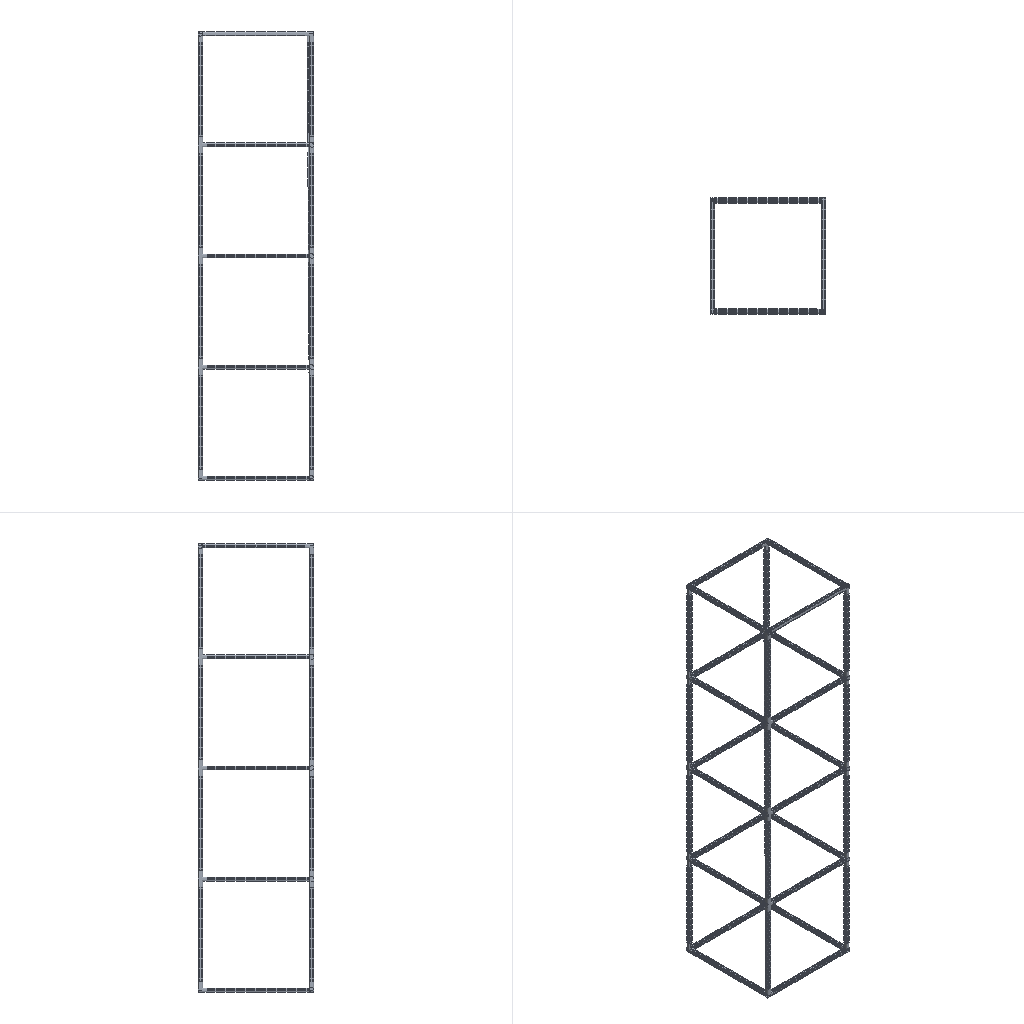Simulation study | ansys workbench
Ansys APDL input file, long lists of numbers shortened:
/batch
/config,noeldb,1     ! force off writing results to database
*get,_wallstrt,active,,time,wall
! ANSYS input file written by Workbench version 2022 R1
! File used for geometry attach:
/title,jiazi--__ (B5)
! ****** Begin Custom Load Command Snippet ******
/COM, ACT Extensions:
/COM,     LSDYNA, 2021.1
/COM,
! ****** End   Custom Load Command Snippet ******
*DIM,_wb_ProjectScratch_dir,string,248
_wb_ProjectScratch_dir(1) = ''
*DIM,_wb_SolverFiles_dir,string,248
_wb_SolverFiles_dir(1) = ''
*DIM,_wb_userfiles_dir,string,248
_wb_userfiles_dir(1) = ''
/com,--- Data in consistent NMM units. See Solving Units in the help system for more information.
/units,MPA
/nopr
/wb,file,start              !  signify a WB generated input file
/prep7
! Turn off shape checking because checks already performed inside WB mesher.
! See help system for more information.
SHPP,OFF,,NOWARN
/nolist
etcon,set             ! allow ANSYS to choose best KEYOP's for 180x elements, resets any applicable keyopt to MAPDL defaults
/com,*********** Nodes for the whole assembly ***********
nblock,3,,145860
(1i9,3e20.9e3)
        1     2.400000000E+02    -2.400000000E+02    -5.000000000E+02
! (132599 more lines like these left out)
-1
/wb,elem,start            !  set before creation of elements
/com,*********** Elements for Body 1 "__-FreeParts|__ 20 X 20 X 2.0(1)[4]" ***********
et,1,186
keyo,1,2,1          ! set full integration on SOLID186
eblock,19,solid,,600
(19i9)
        1        1        1        1        0        0        0        0       20        0     3026    18891    18988    19490    19491    18915    18918    19466    19492
! (1199 more lines like these left out)
-1
/com,*********** Elements for Body 2 "__-FreeParts|__ 20 X 20 X 2.0(1)[2]" ***********
et,2,186
keyo,2,2,1          ! set full integration on SOLID186
eblock,19,solid,,600
(19i9)
        2        2        2        2        0        0        0        0       20        0     4826    29922    29929    30704    30678    29925    29928    30703    30702
! (1199 more lines like these left out)
-1
/com,*********** Elements for Body 3 "__-FreeParts|__(__)1[9]" ***********
et,3,186
keyo,3,2,1          ! set full integration on SOLID186
eblock,19,solid,,600
(19i9)
        3        3        3        3        0        0        0        0       20        0     6051    37691    37740    38265    38289    37692    37716    38191    38290
! (1199 more lines like these left out)
-1
/com,*********** Elements for Body 4 "__-FreeParts|__ 20 X 20 X 2.0(2)[4]" ***********
et,4,186
keyo,4,2,1          ! set full integration on SOLID186
eblock,19,solid,,625
(19i9)
        4        4        4        4        0        0        0        0       20        0     5426    33634    33708    34133    34157    33660    33684    34059    34158
! (1249 more lines like these left out)
-1
/com,*********** Elements for Body 5 "__-FreeParts|__ 20 X 20 X 2.0(2)[2]" ***********
et,5,186
keyo,5,2,1          ! set full integration on SOLID186
eblock,19,solid,,600
(19i9)
        5        5        5        5        0        0        0        0       20        0     4226    26347    26350    27048    27049    26348    26349    27024    27123
! (1199 more lines like these left out)
-1
! (19 more sections like these left out)
/wb,elem,end               !  done creating elements
/com,*********** Send User Defined Coordinate System(s) ***********
csys,0
toffst,273.15,  ! Temperature offset from absolute zero
/com,*********** Set Reference Temperature ***********
tref,22.
/wb,mat,start              !  starting to send materials
/com,*********** Send Materials ***********
Temperature = 'TEMP' ! Temperature
MP,DENS,1,7.85e-09,	! tonne mm^-3
MP,ALPX,1,1.2e-05,	! C^-1
MP,C,1,434000000,	! mm^2 s^-2 C^-1
MP,KXX,1,60.5,	! tonne mm s^-3 C^-1
MP,RSVX,1,0.00017,	! ohm mm
MP,EX,1,200000,	! tonne s^-2 mm^-1
MP,NUXY,1,0.3,
MP,MURX,1,10000,
Temperature = 'TEMP' ! Temperature
MP,DENS,2,7.85e-09,	! tonne mm^-3
MP,ALPX,2,1.2e-05,	! C^-1
MP,C,2,434000000,	! mm^2 s^-2 C^-1
MP,KXX,2,60.5,	! tonne mm s^-3 C^-1
MP,RSVX,2,0.00017,	! ohm mm
MP,EX,2,200000,	! tonne s^-2 mm^-1
MP,NUXY,2,0.3,
MP,MURX,2,10000,
Temperature = 'TEMP' ! Temperature
MP,DENS,3,7.85e-09,	! tonne mm^-3
MP,ALPX,3,1.2e-05,	! C^-1
MP,C,3,434000000,	! mm^2 s^-2 C^-1
MP,KXX,3,60.5,	! tonne mm s^-3 C^-1
MP,RSVX,3,0.00017,	! ohm mm
MP,EX,3,200000,	! tonne s^-2 mm^-1
MP,NUXY,3,0.3,
MP,MURX,3,10000,
Temperature = 'TEMP' ! Temperature
MP,DENS,4,7.85e-09,	! tonne mm^-3
MP,ALPX,4,1.2e-05,	! C^-1
MP,C,4,434000000,	! mm^2 s^-2 C^-1
MP,KXX,4,60.5,	! tonne mm s^-3 C^-1
MP,RSVX,4,0.00017,	! ohm mm
MP,EX,4,200000,	! tonne s^-2 mm^-1
MP,NUXY,4,0.3,
MP,MURX,4,10000,
Temperature = 'TEMP' ! Temperature
MP,DENS,5,7.85e-09,	! tonne mm^-3
MP,ALPX,5,1.2e-05,	! C^-1
MP,C,5,434000000,	! mm^2 s^-2 C^-1
MP,KXX,5,60.5,	! tonne mm s^-3 C^-1
MP,RSVX,5,0.00017,	! ohm mm
MP,EX,5,200000,	! tonne s^-2 mm^-1
MP,NUXY,5,0.3,
MP,MURX,5,10000,
Temperature = 'TEMP' ! Temperature
MP,DENS,6,7.85e-09,	! tonne mm^-3
MP,ALPX,6,1.2e-05,	! C^-1
MP,C,6,434000000,	! mm^2 s^-2 C^-1
MP,KXX,6,60.5,	! tonne mm s^-3 C^-1
MP,RSVX,6,0.00017,	! ohm mm
MP,EX,6,200000,	! tonne s^-2 mm^-1
MP,NUXY,6,0.3,
MP,MURX,6,10000,
Temperature = 'TEMP' ! Temperature
MP,DENS,7,7.85e-09,	! tonne mm^-3
MP,ALPX,7,1.2e-05,	! C^-1
MP,C,7,434000000,	! mm^2 s^-2 C^-1
MP,KXX,7,60.5,	! tonne mm s^-3 C^-1
MP,RSVX,7,0.00017,	! ohm mm
MP,EX,7,200000,	! tonne s^-2 mm^-1
MP,NUXY,7,0.3,
MP,MURX,7,10000,
Temperature = 'TEMP' ! Temperature
MP,DENS,8,7.85e-09,	! tonne mm^-3
MP,ALPX,8,1.2e-05,	! C^-1
MP,C,8,434000000,	! mm^2 s^-2 C^-1
MP,KXX,8,60.5,	! tonne mm s^-3 C^-1
MP,RSVX,8,0.00017,	! ohm mm
MP,EX,8,200000,	! tonne s^-2 mm^-1
MP,NUXY,8,0.3,
MP,MURX,8,10000,
Temperature = 'TEMP' ! Temperature
MP,DENS,9,7.85e-09,	! tonne mm^-3
MP,ALPX,9,1.2e-05,	! C^-1
MP,C,9,434000000,	! mm^2 s^-2 C^-1
MP,KXX,9,60.5,	! tonne mm s^-3 C^-1
MP,RSVX,9,0.00017,	! ohm mm
MP,EX,9,200000,	! tonne s^-2 mm^-1
! (137 more lines like these left out)
/wb,mat,end                !  done sending materials
!************************* Model Summary ********************
!__-FreeParts|__ 20 X 20 X 2.0(1)[4],	结构钢,	matid,	1
!__-FreeParts|__ 20 X 20 X 2.0(1)[2],	结构钢,	matid,	2
!__-FreeParts|__(__)1[9],	结构钢,	matid,	3
!__-FreeParts|__ 20 X 20 X 2.0(2)[4],	结构钢,	matid,	4
!__-FreeParts|__ 20 X 20 X 2.0(2)[2],	结构钢,	matid,	5
!__-FreeParts|__(__)1[3],	结构钢,	matid,	6
!__-FreeParts|__(__)1[8],	结构钢,	matid,	7
!__-FreeParts|__ 20 X 20 X 2.0(1)[3],	结构钢,	matid,	8
!__-FreeParts|__(__)1[12],	结构钢,	matid,	9
!__-FreeParts|__(__)1[2],	结构钢,	matid,	10
!__-FreeParts|__(__)1[4],	结构钢,	matid,	11
!__-FreeParts|__ 20 X 20 X 2.0(3)[3],	结构钢,	matid,	12
!__-FreeParts|__ 20 X 20 X 2.0(2)[3],	结构钢,	matid,	13
!__-FreeParts|__ 20 X 20 X 2.0(1)[1],	结构钢,	matid,	14
!__-FreeParts|__(__)1[10],	结构钢,	matid,	15
!__-FreeParts|__(__)1[6],	结构钢,	matid,	16
!__-FreeParts|__ 20 X 20 X 2.0(3)[4],	结构钢,	matid,	17
!__-FreeParts|__ 20 X 20 X 2.0(3)[1],	结构钢,	matid,	18
!__-FreeParts|__ 20 X 20 X 2.0(2)[1],	结构钢,	matid,	19
!__-FreeParts|__(__)1[5],	结构钢,	matid,	20
!__-FreeParts|__(__)1[1],	结构钢,	matid,	21
!__-FreeParts|__ 20 X 20 X 2.0(3)[2],	结构钢,	matid,	22
!__-FreeParts|__(__)1[11],	结构钢,	matid,	23
!__-FreeParts|__(__)1[7],	结构钢,	matid,	24
!************************* End Model Summary ********************
! get the diagonal of the bounding box. Needed later for other things
*get,_xmin,node,,mnloc,x
*get,_ymin,node,,mnloc,y
*get,_zmin,node,,mnloc,z
*get,_xmax,node,,mxloc,x
*get,_ymax,node,,mxloc,y
*get,_zmax,node,,mxloc,z
_ASMDIAG=(_xmax-_xmin)*(_xmax-_xmin)+(_ymax-_ymin)*(_ymax-_ymin)+(_zmax-_zmin)*(_zmax-_zmin)
_ASMDIAG=SQRT(_ASMDIAG)
/wb,contact,start          !  starting to send contact
/com,*********** Create Contact "接触区域" ***********
/com,            Real Constant Set For Above Contact Is 26 & 25
*set,tid,26
*set,cid,25
r,tid
r,cid
et,tid,170
et,cid,174
eblock,10,,,12
(15i9)
    58871       26       26       26        0    19515    19516    18709    18710    21988    19772    19770    19775
! (11 more lines like these left out)
-1
eblock,10,,,12
(15i9)
    58883       25       25       25        0    19515    19516    18709    18710    21988    19772    19770    19775
! (11 more lines like these left out)
-1
eblock,10,,,25
(15i9)
    58895       25       26       25        0    15157    15156    15658    15658    16950    16951    15658    16953
! (24 more lines like these left out)
-1
eblock,10,,,25
(15i9)
    58920       26       25       26        0    15157    15156    15658    15658    16950    16951    15658    16953
! (24 more lines like these left out)
-1
keyo,cid,8,2               ! auto create asymmetric contact (from Program Controlled setting)
keyo,cid,10,0              ! adjust contact stiffness each NR iteration (from Program Controlled setting)
keyo,cid,12,5              ! bonded always
keyo,cid,18,1              ! small sliding turned on by application
keyo,cid,2,0               ! augmented Lagrange (from Program Controlled setting)
keyo,cid,4,0               ! on Gauss point (from Program Controlled setting)
keyo,cid,9,1               ! ignore initial gaps/penetration
keyo,cid,7,0               ! No Prediction
rmod,tid,3,10.      ! FKN
rmod,tid,5,0.       ! ICONT
rmod,tid,6,0.       ! PINB
rmod,tid,10,0.      ! CNOF
rmod,tid,12,0.      ! FKT
rmod,tid,36,95      ! WB DSID
rmod,cid,3,10.      ! FKN
rmod,cid,5,0.       ! ICONT
rmod,cid,6,0.       ! PINB
rmod,cid,10,0.      ! CNOF
rmod,cid,12,0.      ! FKT
rmod,cid,36,95      ! WB DSID
/com,*********** Create Contact "接触区域 2" ***********
/com,            Real Constant Set For Above Contact Is 28 & 27
*set,tid,28
*set,cid,27
r,tid
r,cid
et,tid,170
et,cid,174
eblock,10,,,64
(15i9)
    58945       28       28       28        0    18865    18810    18807    18864    20079    20069    20070    20235
! (63 more lines like these left out)
-1
eblock,10,,,64
(15i9)
    59009       27       27       27        0    18865    18810    18807    18864    20079    20069    20070    20235
! (63 more lines like these left out)
-1
eblock,10,,,64
(15i9)
    59073       27       28       27        0    52458    52257    52256    52255    56363    56360    56358    56359
! (63 more lines like these left out)
-1
eblock,10,,,64
(15i9)
    59137       28       27       28        0    52458    52257    52256    52255    56363    56360    56358    56359
! (63 more lines like these left out)
-1
keyo,cid,8,2               ! auto create asymmetric contact (from Program Controlled setting)
keyo,cid,10,0              ! adjust contact stiffness each NR iteration (from Program Controlled setting)
keyo,cid,12,5              ! bonded always
keyo,cid,18,1              ! small sliding turned on by application
keyo,cid,2,0               ! augmented Lagrange (from Program Controlled setting)
keyo,cid,4,0               ! on Gauss point (from Program Controlled setting)
keyo,cid,9,1               ! ignore initial gaps/penetration
keyo,cid,7,0               ! No Prediction
rmod,tid,3,10.      ! FKN
rmod,tid,5,0.       ! ICONT
rmod,tid,6,0.       ! PINB
rmod,tid,10,0.      ! CNOF
rmod,tid,12,0.      ! FKT
rmod,tid,36,98      ! WB DSID
rmod,cid,3,10.      ! FKN
rmod,cid,5,0.       ! ICONT
rmod,cid,6,0.       ! PINB
rmod,cid,10,0.      ! CNOF
rmod,cid,12,0.      ! FKT
rmod,cid,36,98      ! WB DSID
/com,*********** Create Contact "接触区域 3" ***********
/com,            Real Constant Set For Above Contact Is 30 & 29
*set,tid,30
*set,cid,29
r,tid
r,cid
et,tid,170
et,cid,174
eblock,10,,,24
(15i9)
    59201       30       30       30        0    18814    18813    19590    19590    20085    20087    19590    20089
! (23 more lines like these left out)
-1
eblock,10,,,24
(15i9)
    59225       29       29       29        0    18814    18813    19590    19590    20085    20087    19590    20089
! (23 more lines like these left out)
-1
eblock,10,,,12
(15i9)
    59249       29       30       29        0    11954    11951    11950    11955    14448    14445    14446    14452
! (11 more lines like these left out)
-1
eblock,10,,,12
(15i9)
    59261       30       29       30        0    11954    11951    11950    11955    14448    14445    14446    14452
! (11 more lines like these left out)
-1
keyo,cid,8,2               ! auto create asymmetric contact (from Program Controlled setting)
keyo,cid,10,0              ! adjust contact stiffness each NR iteration (from Program Controlled setting)
keyo,cid,12,5              ! bonded always
keyo,cid,18,1              ! small sliding turned on by application
keyo,cid,2,0               ! augmented Lagrange (from Program Controlled setting)
keyo,cid,4,0               ! on Gauss point (from Program Controlled setting)
keyo,cid,9,1               ! ignore initial gaps/penetration
keyo,cid,7,0               ! No Prediction
rmod,tid,3,10.      ! FKN
rmod,tid,5,0.       ! ICONT
rmod,tid,6,0.       ! PINB
rmod,tid,10,0.      ! CNOF
rmod,tid,12,0.      ! FKT
rmod,tid,36,101     ! WB DSID
rmod,cid,3,10.      ! FKN
rmod,cid,5,0.       ! ICONT
rmod,cid,6,0.       ! PINB
rmod,cid,10,0.      ! CNOF
rmod,cid,12,0.      ! FKT
rmod,cid,36,101     ! WB DSID
/com,*********** Create Contact "接触区域 4" ***********
/com,            Real Constant Set For Above Contact Is 32 & 31
*set,tid,32
*set,cid,31
r,tid
r,cid
et,tid,170
et,cid,174
eblock,10,,,24
(15i9)
    59273       32       32       32        0    18814    18813    19590    19590    20085    20087    19590    20089
! (23 more lines like these left out)
-1
eblock,10,,,24
(15i9)
    59297       31       31       31        0    18814    18813    19590    19590    20085    20087    19590    20089
! (23 more lines like these left out)
-1
eblock,10,,,12
(15i9)
    59321       31       32       31        0    90084    89983    89982    90083    96575    96572    96573    96873
! (11 more lines like these left out)
-1
eblock,10,,,12
(15i9)
    59333       32       31       32        0    90084    89983    89982    90083    96575    96572    96573    96873
! (11 more lines like these left out)
-1
keyo,cid,8,2               ! auto create asymmetric contact (from Program Controlled setting)
keyo,cid,10,0              ! adjust contact stiffness each NR iteration (from Program Controlled setting)
keyo,cid,12,5              ! bonded always
keyo,cid,18,1              ! small sliding turned on by application
keyo,cid,2,0               ! augmented Lagrange (from Program Controlled setting)
keyo,cid,4,0               ! on Gauss point (from Program Controlled setting)
keyo,cid,9,1               ! ignore initial gaps/penetration
keyo,cid,7,0               ! No Prediction
rmod,tid,3,10.      ! FKN
rmod,tid,5,0.       ! ICONT
rmod,tid,6,0.       ! PINB
rmod,tid,10,0.      ! CNOF
rmod,tid,12,0.      ! FKT
rmod,tid,36,104     ! WB DSID
rmod,cid,3,10.      ! FKN
rmod,cid,5,0.       ! ICONT
rmod,cid,6,0.       ! PINB
rmod,cid,10,0.      ! CNOF
rmod,cid,12,0.      ! FKT
rmod,cid,36,104     ! WB DSID
/com,*********** Create Contact "接触区域 5" ***********
/com,            Real Constant Set For Above Contact Is 34 & 33
*set,tid,34
*set,cid,33
r,tid
r,cid
et,tid,170
et,cid,174
eblock,10,,,24
(15i9)
    59345       34       34       34        0    30401    30400    30802    30802    32604    32605    30802    32607
! (23 more lines like these left out)
-1
eblock,10,,,24
(15i9)
    59369       33       33       33        0    30401    30400    30802    30802    32604    32605    30802    32607
! (23 more lines like these left out)
-1
eblock,10,,,12
(15i9)
    59393       33       34       33        0    15710    15707    15706    15711    18332    18330    18331    18336
! (11 more lines like these left out)
-1
eblock,10,,,12
(15i9)
    59405       34       33       34        0    15710    15707    15706    15711    18332    18330    18331    18336
! (11 more lines like these left out)
-1
keyo,cid,8,2               ! auto create asymmetric contact (from Program Controlled setting)
keyo,cid,10,0              ! adjust contact stiffness each NR iteration (from Program Controlled setting)
keyo,cid,12,5              ! bonded always
keyo,cid,18,1              ! small sliding turned on by application
keyo,cid,2,0               ! augmented Lagrange (from Program Controlled setting)
keyo,cid,4,0               ! on Gauss point (from Program Controlled setting)
keyo,cid,9,1               ! ignore initial gaps/penetration
keyo,cid,7,0               ! No Prediction
rmod,tid,3,10.      ! FKN
rmod,tid,5,0.       ! ICONT
rmod,tid,6,0.       ! PINB
rmod,tid,10,0.      ! CNOF
rmod,tid,12,0.      ! FKT
rmod,tid,36,107     ! WB DSID
rmod,cid,3,10.      ! FKN
rmod,cid,5,0.       ! ICONT
rmod,cid,6,0.       ! PINB
rmod,cid,10,0.      ! CNOF
rmod,cid,12,0.      ! FKT
rmod,cid,36,107     ! WB DSID
! (55 more sections like these left out)
/wb,contact,end            !  done creating contacts
/golist
/wb,load,start             !  starting to send loads
/gst,on,on
fini
*get,_numnode,node,0,count
*get,_numelem,elem,0,count
*get, _MAXELEMNUM, elem, 0, NUM, MAX
*get, _MAXNODENUM, node, 0, NUM, MAX
*get, _MAXELEMTYPE, etyp, 0, NUM, MAX
*get, _MAXREALCONST, real, 0, NUM, MAX
/go
/wb,load,end               !  done creating loads
/com,--- Number of total nodes = %_numnode%
/com,--- Number of contact elements = 9690
/com,--- Number of spring elements = 0
/com,--- Number of bearing elements = 0
/com,--- Number of solid elements = 21674
/com,--- Number of condensed parts = 0
/com,--- Number of total elements = %_numelem%
*get,_wallbsol,active,,time,wall
/solu
antype,2                   ! modal analysis
_thickRatio=  0     ! Ratio of thick parts in the model
modopt,lanb,6
outres,erase
outres,all,none
outres,nsol,all
outres,etmp,all
mxpand                    ! default expand in case of complex solution
dmpopt,esav,no
dmpopt,emat,no
dmpopt,full,no
! *********** WB SOLVE COMMAND ***********
! check interactive state
*get,ANSINTER_,active,,int
*if,ANSINTER_,ne,0,then
/eof
*endif
solve
/com *************** Write FE CONNECTORS *********
CEWRITE,file,ce,,INTE
*get,_nmodalsolproc,active,0,numcpu
fini
/nopr
*get,_numnode,node,0,count
*get,_numelem,elem,0,count
*get, _MAXELEMNUM, elem, 0, NUM, MAX
*get, _MAXNODENUM, node, 0, NUM, MAX,,,INTERNAL
*get, _MAXELEMTYPE, etyp, 0, NUM, MAX
*get, _MAXREALCONST, real, 0, NUM, MAX
/gopr
*get,_wallasol,active,,time,wall
/post1
/nopr
*dim,_direction,CHAR,6,1
_direction(1) = 'X'
_direction(2) = 'Y'
_direction(3) = 'Z'
_direction(4) = 'ROTX'
_direction(5) = 'ROTY'
_direction(6) = 'ROTZ'
*get,_lastLS,active,0,set,LSTP
*get,_beginset,active,0,set,nset,first,_lastLS
*get,_endset,active,0,set,nset,last,_lastLS
_nummodes = 0
*if,_endset,gt,0,then
_nummodes = _endset - _beginset + 1
*endif
*do,i_mode,1,_nummodes
   *do,j_component,1,6
			*get,PFACT_%i_mode%_%j_component%,MODE,%i_mode%,PFACT,,DIREC,_direction(%j_component%)
   *enddo
*enddo
*dim,_tmdirection,CHAR,6,1
_tmdirection(1) = 'X'
_tmdirection(2) = 'Y'
_tmdirection(3) = 'Z'
_tmdirection(4) = 'X'
_tmdirection(5) = 'Y'
_tmdirection(6) = 'Z'
*do,j_component,1,6
    *if,j_component,gt,3,then
        *get,TOTALMASS_%j_component%,ELEM,0,IOR,_tmdirection(%j_component%)
    *else
        *get,TOTALMASS_%j_component%,ELEM,0,MTOT,_tmdirection(%j_component%)
    *endif
*enddo
/gopr
xmlo,ENCODING,ISO-8859-1
xmlo,parm
/xml,parm,xml
fini
/gopr
*get,_walldone,active,,time,wall
_preptime=(_wallbsol-_wallstrt)*3600
_solvtime=(_wallasol-_wallbsol)*3600
_posttime=(_walldone-_wallasol)*3600
_totaltim=(_walldone-_wallstrt)*3600
*get,_dlbratio,active,0,solu,dlbr
*get,_combtime,active,0,solu,comb
*get,_ssmode,active,0,solu,ssmm
*get,_ndofs,active,0,solu,ndof
/fclean				!clean distributed files
/com,--- Total number of nodes = %_numnode%
/com,--- Total number of elements = %_numelem%
/com,--- Element load balance ratio = %_dlbratio%
/com,--- Time to combine distributed files = %_combtime%
/com,--- Sparse memory mode = %_ssmode%
/com,--- Number of DOF = %_ndofs%
/wb,file,end               ! done with WB generated input